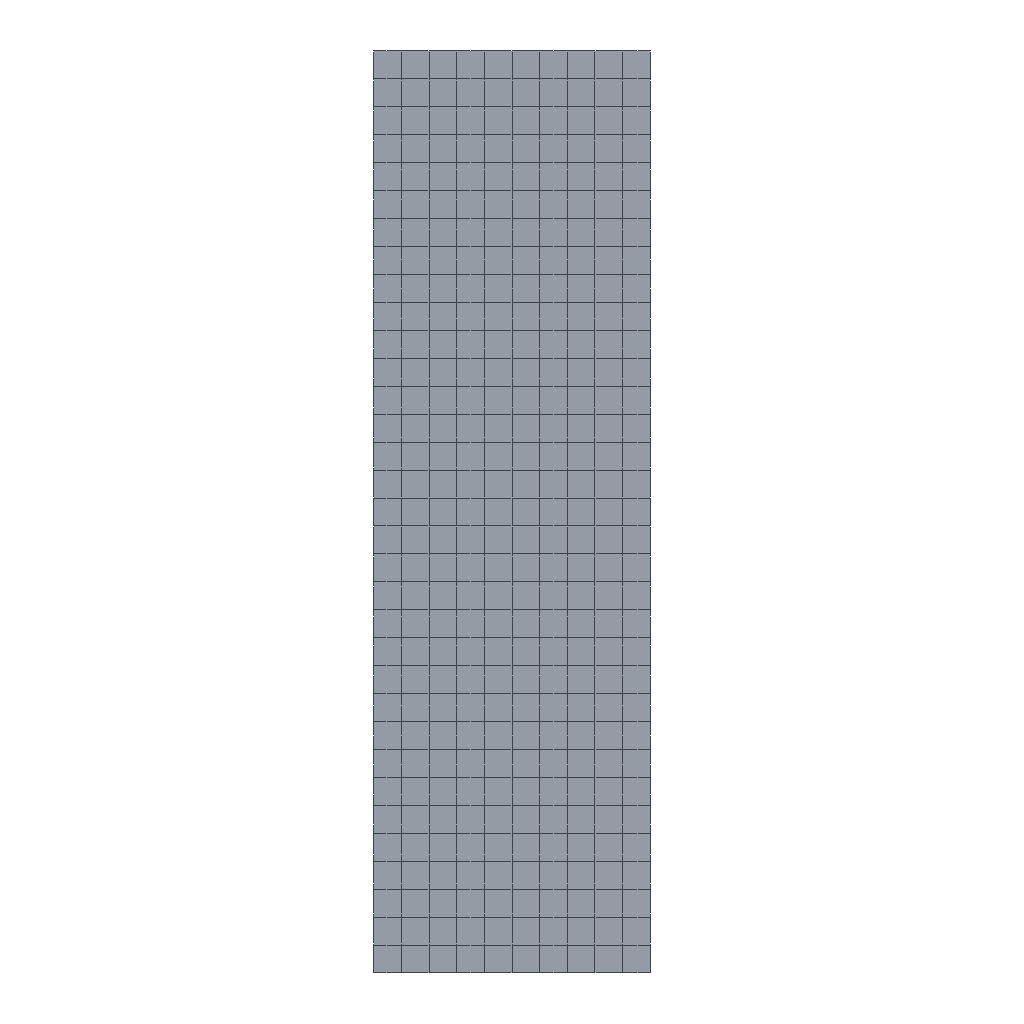Simulation study | abaqus
Set-up summary:
category,name,step,type,value,unit,region
solver,abaqus,,Abaqus/CAE 2024
units,mm-N-s-tonne (MPa),,inferred,E=210000 density=
analysis,Incontact,,static,nlgeom=True; time_period=1
analysis,Press,,static,nlgeom=True; time_period=1
mesh,nodes,,,375
mesh,elements,,,330
element_type,CAX4I,,,330
material,Material-1,,E,210000
material,Material-1,,nu,0.3
material,Material-1,,yield,418
material,Material-1,,behaviors,plastic
section,Material-1,,solid section,,,_PickedSet2
bc,BC-Fix-X,initial,fixed,[dofs=x],,Set-X-Fix
bc,BC-Fix-Y,initial,fixed,[dofs=y],,Set-Y-Fix
bc,BC-Move,Incontact,fixed,"[dofs=rz,x n=2]",,Set-Head-Ref
bc,BC-Move,Incontact,displacement,-5.001 [dofs=y],,Set-Head-Ref
bc,BC-Move,Press,displacement,-25 [dofs=y],,Set-Head-Ref
contact,Int-1,initial,contact pair surface to surface,interaction=IntProp-1,,Surf-Specimen / Head-1.Surf-Head
constraint,rigid body,,,1
Abaqus input file, long lists of numbers shortened:
*Heading
** Job name: deck Model name: Model-1
** Generated by: Abaqus/CAE 2024
*Preprint, echo=NO, model=NO, history=NO, contact=NO
**
** PARTS
**
*Part, name=Head
*End Part
**
*Part, name=Specimen
*Node
      1,          15.,          50.
      2,         13.5,          50.
** (372 more lines like these left out)
*Element, type=CAX4I
  1,   1,   2,  13,  12
  2,   2,   3,  14,  13
** (328 more lines like these left out)
*Nset, nset=_PickedSet2, internal, generate
   1,  374,    1
*Elset, elset=_PickedSet2, internal, generate
   1,  330,    1
** Section: Section-1
*Solid Section, elset=_PickedSet2, material=Material-1
1.,
*End Part
**
**
** ASSEMBLY
**
*Assembly, name=Assembly
**
*Instance, name=Head-1, part=Head
*Node
      1,          15.,          55.,           0.
*Nset, nset=Head-1-RefPt_, internal
1,
*Surface, type=SEGMENTS, name=Surf-Head
START,          30.,          55.
 LINE,           0.,          55.
*Rigid Body, ref node=Head-1-RefPt_, analytical surface=Surf-Head
*End Instance
**
*Instance, name=Specimen-1, part=Specimen
*End Instance
**
*Nset, nset=Set-Head-Ref, instance=Head-1
 1,
*Nset, nset=Set-X-Fix, instance=Specimen-1, generate
  11,  374,   11
*Elset, elset=Set-X-Fix, instance=Specimen-1, generate
  10,  330,   10
*Nset, nset=Set-Y-Fix, instance=Specimen-1, generate
 364,  374,    1
*Elset, elset=Set-Y-Fix, instance=Specimen-1, generate
 321,  330,    1
*Elset, elset=_Set-X-Fix_S2, internal, instance=Specimen-1, generate
  10,  330,   10
*Surface, type=ELEMENT, name=Set-X-Fix
_Set-X-Fix_S2, S2
*Elset, elset=_Set-Y-Fix_S3, internal, instance=Specimen-1, generate
 321,  330,    1
*Surface, type=ELEMENT, name=Set-Y-Fix
_Set-Y-Fix_S3, S3
*Elset, elset=_Surf-Specimen_S1, internal, instance=Specimen-1, generate
  1,  10,   1
*Surface, type=ELEMENT, name=Surf-Specimen
_Surf-Specimen_S1, S1
*End Assembly
**
** MATERIALS
**
*Material, name=Material-1
*Elastic
210000., 0.3
*Plastic
 418.,      0.
 500., 0.01581
 605., 0.02983
 695.,   0.056
 780.,   0.095
 829.,    0.15
 882.,    0.25
 908.,    0.35
 921.,    0.45
 932.,    0.55
 955.,    0.65
 988.,    0.75
1040.,    0.85
**
** INTERACTION PROPERTIES
**
*Surface Interaction, name=IntProp-1
1.,
**
** BOUNDARY CONDITIONS
**
** Name: BC-Fix-X Type: Displacement/Rotation
*Boundary
Set-X-Fix, 1, 1
** Name: BC-Fix-Y Type: Displacement/Rotation
*Boundary
Set-Y-Fix, 2, 2
**
** INTERACTIONS
**
** Interaction: Int-1
*Contact Pair, interaction=IntProp-1, type=SURFACE TO SURFACE
Surf-Specimen, Head-1.Surf-Head
** ----------------------------------------------------------------
**
** STEP: Incontact
**
*Step, name=Incontact, nlgeom=YES
*Static
1., 1., 1e-05, 1.
**
** BOUNDARY CONDITIONS
**
** Name: BC-Move Type: Displacement/Rotation
*Boundary
Set-Head-Ref, 1, 1
Set-Head-Ref, 2, 2, -5.001
Set-Head-Ref, 6, 6
**
** OUTPUT REQUESTS
**
*Restart, write, frequency=0
*Print, solve=NO
**
** FIELD OUTPUT: F-Output-1
**
*Output, field
*Node Output
CF, RF, U
*Element Output, directions=YES
LE, MISESMAX, PE, PEEQ, PEMAG, S
*Contact Output
CDISP, CSTRESS
*NODE PRINT,NSET=Set-Head-Ref
RF,
**
** HISTORY OUTPUT: H-Output-1
**
*Output, history, variable=PRESELECT
*End Step
** ----------------------------------------------------------------
**
** STEP: Press
**
*Step, name=Press, nlgeom=YES
*Static
0.05, 1., 1e-05, 0.05
**
** BOUNDARY CONDITIONS
**
** Name: BC-Move Type: Displacement/Rotation
*Boundary
Set-Head-Ref, 2, 2, -25.
**
** OUTPUT REQUESTS
**
*Restart, write, frequency=0
**
** FIELD OUTPUT: F-Output-1
**
*Output, field
*Node Output
CF, RF, U
*Element Output, directions=YES
LE, MISESMAX, PE, PEEQ, PEMAG, S
*Contact Output
CDISP, CSTRESS
**
** HISTORY OUTPUT: H-Output-1
**
*Output, history, variable=PRESELECT
*End Step
Results summary:
result,odb.job_status,,,JOB_STATUS_COMPLETED_SUCCESSFULLY,"consistent, unstated (Abaqus has no unit system)"
result,steps[0].procedure,Incontact,,*STATIC,"consistent, unstated (Abaqus has no unit system)"
result,steps[0].time_period,Incontact,,1,"consistent, unstated (Abaqus has no unit system)"
result,steps[0].n_frames,Incontact,,2,"consistent, unstated (Abaqus has no unit system)"
result,steps[0].last_frame.id,Incontact,,1,"consistent, unstated (Abaqus has no unit system)"
result,steps[0].last_frame.value,Incontact,,1,"consistent, unstated (Abaqus has no unit system)"
result,steps[0].last_frame.description,Incontact,,Increment      1: Step Time =    1.000,"consistent, unstated (Abaqus has no unit system)"
result,steps[0].completed,Incontact,,True,"consistent, unstated (Abaqus has no unit system)"
result,steps[0].max_U_magnitude,Incontact,,5.001,"consistent, unstated (Abaqus has no unit system)"
result,steps[0].max_S_mises,Incontact,,4.176,"consistent, unstated (Abaqus has no unit system)"
result,steps[0].RF_sum[1],Incontact,,1.09062e-10,"consistent, unstated (Abaqus has no unit system)"
result,steps[0].RF_sum[2],Incontact,,0.04257,"consistent, unstated (Abaqus has no unit system)"
result,steps[0].diagnostic.n_increments,Incontact,,1,"consistent, unstated (Abaqus has no unit system)"
result,steps[1].procedure,Press,,*STATIC,"consistent, unstated (Abaqus has no unit system)"
result,steps[1].time_period,Press,,1,"consistent, unstated (Abaqus has no unit system)"
result,steps[1].n_frames,Press,,21,"consistent, unstated (Abaqus has no unit system)"
result,steps[1].last_frame.id,Press,,20,"consistent, unstated (Abaqus has no unit system)"
result,steps[1].last_frame.value,Press,,1,"consistent, unstated (Abaqus has no unit system)"
result,steps[1].last_frame.description,Press,,Increment     20: Step Time =    1.000,"consistent, unstated (Abaqus has no unit system)"
result,steps[1].completed,Press,,True,"consistent, unstated (Abaqus has no unit system)"
result,steps[1].max_U_magnitude,Press,,25,"consistent, unstated (Abaqus has no unit system)"
result,steps[1].max_S_mises,Press,,927.198,"consistent, unstated (Abaqus has no unit system)"
result,steps[1].RF_sum[1],Press,,0.007453,"consistent, unstated (Abaqus has no unit system)"
result,steps[1].RF_sum[2],Press,,-1.753,"consistent, unstated (Abaqus has no unit system)"
result,steps[1].diagnostic.n_increments,Press,,20,"consistent, unstated (Abaqus has no unit system)"